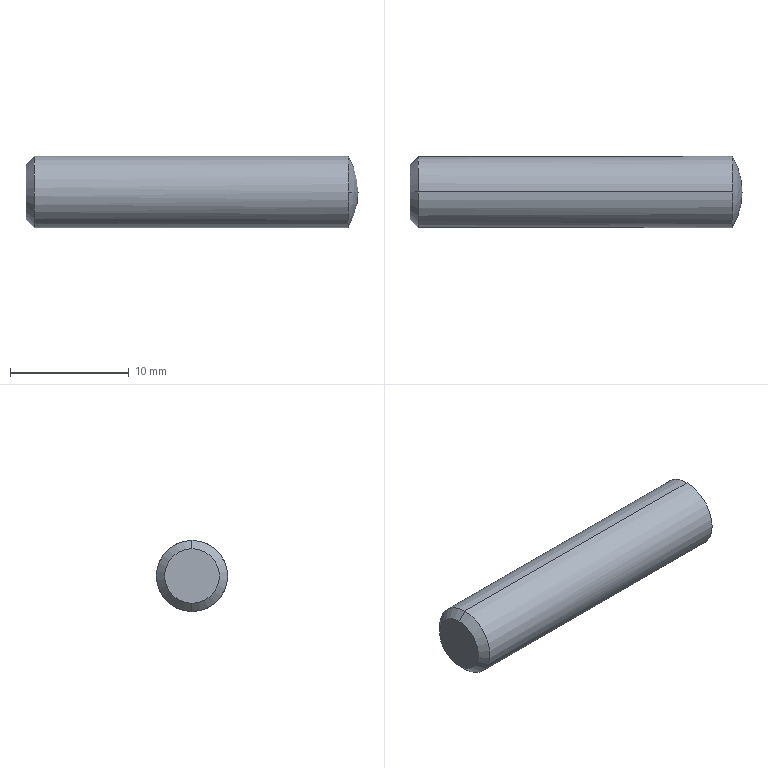Part | SolidWorks | features BaseBody 1 | 1 solid | 7 faces | box 28 x 6 x 6 mm | volume 776.33 mm3 | cylinder 2 | sphere 2 | cone 2 | plane 1 | commonest cylinder face diameters 6 x2
STEP:
#1=CARTESIAN_POINT('',(7.233,-74.104,-8.75));
#2=VERTEX_POINT('',#1);
#3=CARTESIAN_POINT('',(7.233,-71.104,-5.75));
#4=VERTEX_POINT('',#3);
#5=CARTESIAN_POINT('',(7.233,-71.104,-8.75));
#6=DIRECTION('',(-1.,0.,0.));
#7=DIRECTION('',(0.,0.,-1.));
#8=AXIS2_PLACEMENT_3D('',#5,#6,#7);
#9=CIRCLE('',#8,3.);
#10=EDGE_CURVE('',#2,#4,#9,.T.);
#11=ORIENTED_EDGE('',*,*,#10,.T.);
#12=CARTESIAN_POINT('',(-19.263,-71.104,-5.75));
#13=VERTEX_POINT('',#12);
#14=CARTESIAN_POINT('',(-19.963,-71.104,-5.75));
#15=DIRECTION('',(-1.,0.,0.));
#16=VECTOR('',#15,1000.);
#17=LINE('',#14,#16);
#18=EDGE_CURVE('',#4,#13,#17,.T.);
#19=ORIENTED_EDGE('',*,*,#18,.T.);
#20=CARTESIAN_POINT('',(-19.263,-71.104,-11.75));
#21=VERTEX_POINT('',#20);
#22=CARTESIAN_POINT('',(-19.263,-71.104,-8.75));
#23=DIRECTION('',(1.,0.,0.));
#24=DIRECTION('',(0.,0.,-1.));
#25=AXIS2_PLACEMENT_3D('',#22,#23,#24);
#26=CIRCLE('',#25,3.);
#27=EDGE_CURVE('',#13,#21,#26,.T.);
#28=ORIENTED_EDGE('',*,*,#27,.T.);
#29=CARTESIAN_POINT('',(7.233,-71.104,-11.75));
#30=VERTEX_POINT('',#29);
#31=CARTESIAN_POINT('',(-19.963,-71.104,-11.75));
#32=DIRECTION('',(-1.,0.,0.));
#33=VECTOR('',#32,1000.);
#34=LINE('',#31,#33);
#35=EDGE_CURVE('',#30,#21,#34,.T.);
#36=ORIENTED_EDGE('',*,*,#35,.F.);
#37=CARTESIAN_POINT('',(7.233,-71.104,-8.75));
#38=DIRECTION('',(-1.,0.,0.));
#39=DIRECTION('',(0.,0.,-1.));
#40=AXIS2_PLACEMENT_3D('',#37,#38,#39);
#41=CIRCLE('',#40,3.);
#42=EDGE_CURVE('',#30,#2,#41,.T.);
#43=ORIENTED_EDGE('',*,*,#42,.T.);
#44=EDGE_LOOP('',(#11,#19,#28,#36,#43));
#45=FACE_OUTER_BOUND('',#44,.T.);
#46=CARTESIAN_POINT('',(-19.963,-71.104,-8.75));
#47=DIRECTION('',(-1.,0.,0.));
#48=DIRECTION('',(0.,0.,-1.));
#49=AXIS2_PLACEMENT_3D('',#46,#47,#48);
#50=CYLINDRICAL_SURFACE('',#49,3.);
#51=ADVANCED_FACE('',(#45),#50,.T.);
#52=CARTESIAN_POINT('',(8.037,-71.104,-8.75));
#53=VERTEX_POINT('',#52);
#54=CARTESIAN_POINT('',(2.037,-71.104,-8.75));
#55=DIRECTION('',(0.,0.,-1.));
#56=DIRECTION('',(-1.,0.,0.));
#57=AXIS2_PLACEMENT_3D('',#54,#55,#56);
#58=CIRCLE('',#57,6.);
#59=EDGE_CURVE('',#53,#2,#58,.T.);
#60=ORIENTED_EDGE('',*,*,#59,.F.);
#61=CARTESIAN_POINT('',(7.233,-68.104,-8.75));
#62=VERTEX_POINT('',#61);
#63=CARTESIAN_POINT('',(2.037,-71.104,-8.75));
#64=DIRECTION('',(0.,0.,1.));
#65=DIRECTION('',(0.,-1.,0.));
#66=AXIS2_PLACEMENT_3D('',#63,#64,#65);
#67=CIRCLE('',#66,6.);
#68=EDGE_CURVE('',#53,#62,#67,.T.);
#69=ORIENTED_EDGE('',*,*,#68,.T.);
#70=CARTESIAN_POINT('',(7.233,-71.104,-8.75));
#71=DIRECTION('',(-1.,0.,0.));
#72=DIRECTION('',(0.,0.,-1.));
#73=AXIS2_PLACEMENT_3D('',#70,#71,#72);
#74=CIRCLE('',#73,3.);
#75=EDGE_CURVE('',#4,#62,#74,.T.);
#76=ORIENTED_EDGE('',*,*,#75,.F.);
#77=ORIENTED_EDGE('',*,*,#10,.F.);
#78=EDGE_LOOP('',(#60,#69,#76,#77));
#79=FACE_OUTER_BOUND('',#78,.T.);
#80=CARTESIAN_POINT('',(2.037,-71.104,-8.75));
#81=DIRECTION('',(0.,0.,1.));
#82=DIRECTION('',(0.,-1.,0.));
#83=AXIS2_PLACEMENT_3D('',#80,#81,#82);
#84=SPHERICAL_SURFACE('',#83,6.);
#85=ADVANCED_FACE('',(#79),#84,.T.);
#86=CARTESIAN_POINT('',(-19.963,-71.104,-11.05));
#87=VERTEX_POINT('',#86);
#88=CARTESIAN_POINT('',(-19.963,-71.104,-6.45));
#89=VERTEX_POINT('',#88);
#90=CARTESIAN_POINT('',(-19.963,-71.104,-8.75));
#91=DIRECTION('',(-1.,0.,0.));
#92=DIRECTION('',(0.,0.,-1.));
#93=AXIS2_PLACEMENT_3D('',#90,#91,#92);
#94=CIRCLE('',#93,2.3);
#95=EDGE_CURVE('',#87,#89,#94,.T.);
#96=ORIENTED_EDGE('',*,*,#95,.F.);
#97=CARTESIAN_POINT('',(-19.963,-71.104,-11.05));
#98=DIRECTION('',(0.7071,0.,-0.7071));
#99=VECTOR('',#98,1000.);
#100=LINE('',#97,#99);
#101=EDGE_CURVE('',#87,#21,#100,.T.);
#102=ORIENTED_EDGE('',*,*,#101,.T.);
#103=ORIENTED_EDGE('',*,*,#27,.F.);
#104=CARTESIAN_POINT('',(-19.963,-71.104,-6.45));
#105=DIRECTION('',(0.7071,0.,0.7071));
#106=VECTOR('',#105,1000.);
#107=LINE('',#104,#106);
#108=EDGE_CURVE('',#89,#13,#107,.T.);
#109=ORIENTED_EDGE('',*,*,#108,.F.);
#110=EDGE_LOOP('',(#96,#102,#103,#109));
#111=FACE_OUTER_BOUND('',#110,.T.);
#112=CARTESIAN_POINT('',(-19.963,-71.104,-8.75));
#113=DIRECTION('',(1.,0.,0.));
#114=DIRECTION('',(0.,0.,1.));
#115=AXIS2_PLACEMENT_3D('',#112,#113,#114);
#116=CONICAL_SURFACE('',#115,2.3,0.7854);
#117=ADVANCED_FACE('',(#111),#116,.T.);
#118=ORIENTED_EDGE('',*,*,#101,.F.);
#119=CARTESIAN_POINT('',(-19.963,-71.104,-8.75));
#120=DIRECTION('',(-1.,0.,0.));
#121=DIRECTION('',(0.,0.,-1.));
#122=AXIS2_PLACEMENT_3D('',#119,#120,#121);
#123=CIRCLE('',#122,2.3);
#124=EDGE_CURVE('',#89,#87,#123,.T.);
#125=ORIENTED_EDGE('',*,*,#124,.F.);
#126=ORIENTED_EDGE('',*,*,#108,.T.);
#127=CARTESIAN_POINT('',(-19.263,-71.104,-8.75));
#128=DIRECTION('',(1.,0.,0.));
#129=DIRECTION('',(0.,0.,-1.));
#130=AXIS2_PLACEMENT_3D('',#127,#128,#129);
#131=CIRCLE('',#130,3.);
#132=EDGE_CURVE('',#21,#13,#131,.T.);
#133=ORIENTED_EDGE('',*,*,#132,.F.);
#134=EDGE_LOOP('',(#118,#125,#126,#133));
#135=FACE_OUTER_BOUND('',#134,.T.);
#136=CARTESIAN_POINT('',(-19.963,-71.104,-8.75));
#137=DIRECTION('',(1.,0.,0.));
#138=DIRECTION('',(0.,0.,1.));
#139=AXIS2_PLACEMENT_3D('',#136,#137,#138);
#140=CONICAL_SURFACE('',#139,2.3,0.7854);
#141=ADVANCED_FACE('',(#135),#140,.T.);
#142=ORIENTED_EDGE('',*,*,#68,.F.);
#143=ORIENTED_EDGE('',*,*,#59,.T.);
#144=ORIENTED_EDGE('',*,*,#42,.F.);
#145=CARTESIAN_POINT('',(7.233,-71.104,-8.75));
#146=DIRECTION('',(-1.,0.,0.));
#147=DIRECTION('',(0.,0.,-1.));
#148=AXIS2_PLACEMENT_3D('',#145,#146,#147);
#149=CIRCLE('',#148,3.);
#150=EDGE_CURVE('',#62,#30,#149,.T.);
#151=ORIENTED_EDGE('',*,*,#150,.F.);
#152=EDGE_LOOP('',(#142,#143,#144,#151));
#153=FACE_OUTER_BOUND('',#152,.T.);
#154=CARTESIAN_POINT('',(2.037,-71.104,-8.75));
#155=DIRECTION('',(0.,0.,1.));
#156=DIRECTION('',(0.,-1.,0.));
#157=AXIS2_PLACEMENT_3D('',#154,#155,#156);
#158=SPHERICAL_SURFACE('',#157,6.);
#159=ADVANCED_FACE('',(#153),#158,.T.);
#160=ORIENTED_EDGE('',*,*,#18,.F.);
#161=ORIENTED_EDGE('',*,*,#75,.T.);
#162=ORIENTED_EDGE('',*,*,#150,.T.);
#163=ORIENTED_EDGE('',*,*,#35,.T.);
#164=ORIENTED_EDGE('',*,*,#132,.T.);
#165=EDGE_LOOP('',(#160,#161,#162,#163,#164));
#166=FACE_OUTER_BOUND('',#165,.T.);
#167=CARTESIAN_POINT('',(-19.963,-71.104,-8.75));
#168=DIRECTION('',(-1.,0.,0.));
#169=DIRECTION('',(0.,0.,-1.));
#170=AXIS2_PLACEMENT_3D('',#167,#168,#169);
#171=CYLINDRICAL_SURFACE('',#170,3.);
#172=ADVANCED_FACE('',(#166),#171,.T.);
#173=ORIENTED_EDGE('',*,*,#124,.T.);
#174=ORIENTED_EDGE('',*,*,#95,.T.);
#175=EDGE_LOOP('',(#173,#174));
#176=FACE_OUTER_BOUND('',#175,.T.);
#177=CARTESIAN_POINT('',(-19.963,-71.104,-8.75));
#178=DIRECTION('',(-1.,0.,0.));
#179=DIRECTION('',(0.,0.,1.));
#180=AXIS2_PLACEMENT_3D('',#177,#178,#179);
#181=PLANE('',#180);
#182=ADVANCED_FACE('',(#176),#181,.T.);
#183=CLOSED_SHELL('',(#51,#85,#117,#141,#159,#172,#182));
#184=MANIFOLD_SOLID_BREP('',#183);
#185=CARTESIAN_POINT('',(0.,0.,0.));
#186=DIRECTION('',(0.,0.,1.));
#187=DIRECTION('',(1.,0.,0.));
#188=AXIS2_PLACEMENT_3D('',#185,#186,#187);
#189=(LENGTH_UNIT()NAMED_UNIT(*)SI_UNIT(.MILLI.,.METRE.));
#190=UNCERTAINTY_MEASURE_WITH_UNIT(LENGTH_MEASURE(0.00001),#189,'','');
#191=(NAMED_UNIT(*)PLANE_ANGLE_UNIT()SI_UNIT($,.RADIAN.));
#192=(NAMED_UNIT(*)SI_UNIT($,.STERADIAN.)SOLID_ANGLE_UNIT());
#193=(GEOMETRIC_REPRESENTATION_CONTEXT(3)GLOBAL_UNCERTAINTY_ASSIGNED_CONTEXT((#190))GLOBAL_UNIT_ASSIGNED_CONTEXT((#189,#191,#192))REPRESENTATION_CONTEXT('',''));
#194=ADVANCED_BREP_SHAPE_REPRESENTATION('',(#184,#188),#193);